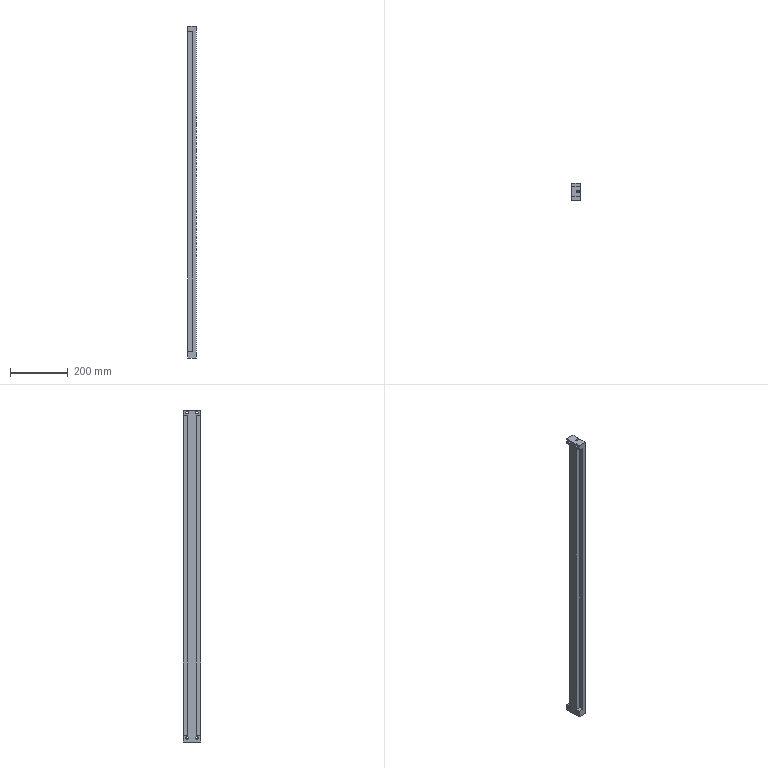Part | STEP file | 750038306 | 1 solid | 26 faces | box 30 x 60 x 1149 mm | volume 1360456 mm3 | plane 18 | cylinder 8 | commonest cylinder face diameters 9 x8
STEP:
#1=CARTESIAN_POINT('',(30.,13.,9.5));
#2=VERTEX_POINT('',#1);
#3=CARTESIAN_POINT('',(30.,13.,18.5));
#4=VERTEX_POINT('',#3);
#5=CARTESIAN_POINT('',(30.,13.,14.));
#6=DIRECTION('',(-1.,0.,0.));
#7=DIRECTION('',(0.,0.,1.));
#8=AXIS2_PLACEMENT_3D('',#5,#6,#7);
#9=CIRCLE('',#8,4.5);
#10=EDGE_CURVE('',#2,#4,#9,.T.);
#11=ORIENTED_EDGE('',*,*,#10,.F.);
#12=CARTESIAN_POINT('',(0.,13.,9.5));
#13=VERTEX_POINT('',#12);
#14=CARTESIAN_POINT('',(33.,13.,9.5));
#15=DIRECTION('',(-1.,0.,0.));
#16=VECTOR('',#15,1000.);
#17=LINE('',#14,#16);
#18=EDGE_CURVE('',#2,#13,#17,.T.);
#19=ORIENTED_EDGE('',*,*,#18,.T.);
#20=CARTESIAN_POINT('',(0.,13.,18.5));
#21=VERTEX_POINT('',#20);
#22=CARTESIAN_POINT('',(0.,13.,14.));
#23=DIRECTION('',(-1.,0.,0.));
#24=DIRECTION('',(0.,0.,1.));
#25=AXIS2_PLACEMENT_3D('',#22,#23,#24);
#26=CIRCLE('',#25,4.5);
#27=EDGE_CURVE('',#13,#21,#26,.T.);
#28=ORIENTED_EDGE('',*,*,#27,.T.);
#29=CARTESIAN_POINT('',(33.,13.,18.5));
#30=DIRECTION('',(-1.,0.,0.));
#31=VECTOR('',#30,1000.);
#32=LINE('',#29,#31);
#33=EDGE_CURVE('',#4,#21,#32,.T.);
#34=ORIENTED_EDGE('',*,*,#33,.F.);
#35=EDGE_LOOP('',(#11,#19,#28,#34));
#36=FACE_OUTER_BOUND('',#35,.T.);
#37=CARTESIAN_POINT('',(33.,13.,14.));
#38=DIRECTION('',(-1.,0.,0.));
#39=DIRECTION('',(0.,0.,1.));
#40=AXIS2_PLACEMENT_3D('',#37,#38,#39);
#41=CYLINDRICAL_SURFACE('',#40,4.5);
#42=ADVANCED_FACE('',(#36),#41,.F.);
#43=CARTESIAN_POINT('',(30.,47.,9.5));
#44=VERTEX_POINT('',#43);
#45=CARTESIAN_POINT('',(30.,47.,18.5));
#46=VERTEX_POINT('',#45);
#47=CARTESIAN_POINT('',(30.,47.,14.));
#48=DIRECTION('',(-1.,0.,0.));
#49=DIRECTION('',(0.,0.,1.));
#50=AXIS2_PLACEMENT_3D('',#47,#48,#49);
#51=CIRCLE('',#50,4.5);
#52=EDGE_CURVE('',#44,#46,#51,.T.);
#53=ORIENTED_EDGE('',*,*,#52,.F.);
#54=CARTESIAN_POINT('',(0.,47.,9.5));
#55=VERTEX_POINT('',#54);
#56=CARTESIAN_POINT('',(33.,47.,9.5));
#57=DIRECTION('',(-1.,0.,0.));
#58=VECTOR('',#57,1000.);
#59=LINE('',#56,#58);
#60=EDGE_CURVE('',#44,#55,#59,.T.);
#61=ORIENTED_EDGE('',*,*,#60,.T.);
#62=CARTESIAN_POINT('',(0.,47.,18.5));
#63=VERTEX_POINT('',#62);
#64=CARTESIAN_POINT('',(0.,47.,14.));
#65=DIRECTION('',(-1.,0.,0.));
#66=DIRECTION('',(0.,0.,1.));
#67=AXIS2_PLACEMENT_3D('',#64,#65,#66);
#68=CIRCLE('',#67,4.5);
#69=EDGE_CURVE('',#55,#63,#68,.T.);
#70=ORIENTED_EDGE('',*,*,#69,.T.);
#71=CARTESIAN_POINT('',(33.,47.,18.5));
#72=DIRECTION('',(-1.,0.,0.));
#73=VECTOR('',#72,1000.);
#74=LINE('',#71,#73);
#75=EDGE_CURVE('',#46,#63,#74,.T.);
#76=ORIENTED_EDGE('',*,*,#75,.F.);
#77=EDGE_LOOP('',(#53,#61,#70,#76));
#78=FACE_OUTER_BOUND('',#77,.T.);
#79=CARTESIAN_POINT('',(33.,47.,14.));
#80=DIRECTION('',(-1.,0.,0.));
#81=DIRECTION('',(0.,0.,1.));
#82=AXIS2_PLACEMENT_3D('',#79,#80,#81);
#83=CYLINDRICAL_SURFACE('',#82,4.5);
#84=ADVANCED_FACE('',(#78),#83,.F.);
#85=CARTESIAN_POINT('',(30.,13.,1135.5));
#86=VERTEX_POINT('',#85);
#87=CARTESIAN_POINT('',(30.,13.,1144.5));
#88=VERTEX_POINT('',#87);
#89=CARTESIAN_POINT('',(30.,13.,1140.));
#90=DIRECTION('',(-1.,0.,0.));
#91=DIRECTION('',(0.,0.,1.));
#92=AXIS2_PLACEMENT_3D('',#89,#90,#91);
#93=CIRCLE('',#92,4.5);
#94=EDGE_CURVE('',#86,#88,#93,.T.);
#95=ORIENTED_EDGE('',*,*,#94,.F.);
#96=CARTESIAN_POINT('',(0.,13.,1135.5));
#97=VERTEX_POINT('',#96);
#98=CARTESIAN_POINT('',(33.,13.,1135.5));
#99=DIRECTION('',(-1.,0.,0.));
#100=VECTOR('',#99,1000.);
#101=LINE('',#98,#100);
#102=EDGE_CURVE('',#86,#97,#101,.T.);
#103=ORIENTED_EDGE('',*,*,#102,.T.);
#104=CARTESIAN_POINT('',(0.,13.,1144.5));
#105=VERTEX_POINT('',#104);
#106=CARTESIAN_POINT('',(0.,13.,1140.));
#107=DIRECTION('',(-1.,0.,0.));
#108=DIRECTION('',(0.,0.,1.));
#109=AXIS2_PLACEMENT_3D('',#106,#107,#108);
#110=CIRCLE('',#109,4.5);
#111=EDGE_CURVE('',#97,#105,#110,.T.);
#112=ORIENTED_EDGE('',*,*,#111,.T.);
#113=CARTESIAN_POINT('',(33.,13.,1144.5));
#114=DIRECTION('',(-1.,0.,0.));
#115=VECTOR('',#114,1000.);
#116=LINE('',#113,#115);
#117=EDGE_CURVE('',#88,#105,#116,.T.);
#118=ORIENTED_EDGE('',*,*,#117,.F.);
#119=EDGE_LOOP('',(#95,#103,#112,#118));
#120=FACE_OUTER_BOUND('',#119,.T.);
#121=CARTESIAN_POINT('',(33.,13.,1140.));
#122=DIRECTION('',(-1.,0.,0.));
#123=DIRECTION('',(0.,0.,1.));
#124=AXIS2_PLACEMENT_3D('',#121,#122,#123);
#125=CYLINDRICAL_SURFACE('',#124,4.5);
#126=ADVANCED_FACE('',(#120),#125,.F.);
#127=CARTESIAN_POINT('',(30.,47.,1135.5));
#128=VERTEX_POINT('',#127);
#129=CARTESIAN_POINT('',(30.,47.,1144.5));
#130=VERTEX_POINT('',#129);
#131=CARTESIAN_POINT('',(30.,47.,1140.));
#132=DIRECTION('',(-1.,0.,0.));
#133=DIRECTION('',(0.,0.,1.));
#134=AXIS2_PLACEMENT_3D('',#131,#132,#133);
#135=CIRCLE('',#134,4.5);
#136=EDGE_CURVE('',#128,#130,#135,.T.);
#137=ORIENTED_EDGE('',*,*,#136,.F.);
#138=CARTESIAN_POINT('',(0.,47.,1135.5));
#139=VERTEX_POINT('',#138);
#140=CARTESIAN_POINT('',(33.,47.,1135.5));
#141=DIRECTION('',(-1.,0.,0.));
#142=VECTOR('',#141,1000.);
#143=LINE('',#140,#142);
#144=EDGE_CURVE('',#128,#139,#143,.T.);
#145=ORIENTED_EDGE('',*,*,#144,.T.);
#146=CARTESIAN_POINT('',(0.,47.,1144.5));
#147=VERTEX_POINT('',#146);
#148=CARTESIAN_POINT('',(0.,47.,1140.));
#149=DIRECTION('',(-1.,0.,0.));
#150=DIRECTION('',(0.,0.,1.));
#151=AXIS2_PLACEMENT_3D('',#148,#149,#150);
#152=CIRCLE('',#151,4.5);
#153=EDGE_CURVE('',#139,#147,#152,.T.);
#154=ORIENTED_EDGE('',*,*,#153,.T.);
#155=CARTESIAN_POINT('',(33.,47.,1144.5));
#156=DIRECTION('',(-1.,0.,0.));
#157=VECTOR('',#156,1000.);
#158=LINE('',#155,#157);
#159=EDGE_CURVE('',#130,#147,#158,.T.);
#160=ORIENTED_EDGE('',*,*,#159,.F.);
#161=EDGE_LOOP('',(#137,#145,#154,#160));
#162=FACE_OUTER_BOUND('',#161,.T.);
#163=CARTESIAN_POINT('',(33.,47.,1140.));
#164=DIRECTION('',(-1.,0.,0.));
#165=DIRECTION('',(0.,0.,1.));
#166=AXIS2_PLACEMENT_3D('',#163,#164,#165);
#167=CYLINDRICAL_SURFACE('',#166,4.5);
#168=ADVANCED_FACE('',(#162),#167,.F.);
#169=CARTESIAN_POINT('',(0.,13.,14.));
#170=DIRECTION('',(-1.,0.,0.));
#171=DIRECTION('',(0.,0.,1.));
#172=AXIS2_PLACEMENT_3D('',#169,#170,#171);
#173=CIRCLE('',#172,4.5);
#174=EDGE_CURVE('',#21,#13,#173,.T.);
#175=ORIENTED_EDGE('',*,*,#174,.F.);
#176=ORIENTED_EDGE('',*,*,#27,.F.);
#177=EDGE_LOOP('',(#175,#176));
#178=FACE_BOUND('',#177,.T.);
#179=CARTESIAN_POINT('',(0.,0.,24.));
#180=VERTEX_POINT('',#179);
#181=CARTESIAN_POINT('',(0.,0.,0.));
#182=VERTEX_POINT('',#181);
#183=CARTESIAN_POINT('',(0.,0.,1149.));
#184=DIRECTION('',(0.,0.,-1.));
#185=VECTOR('',#184,1000.);
#186=LINE('',#183,#185);
#187=EDGE_CURVE('',#180,#182,#186,.T.);
#188=ORIENTED_EDGE('',*,*,#187,.F.);
#189=CARTESIAN_POINT('',(0.,15.,24.));
#190=VERTEX_POINT('',#189);
#191=CARTESIAN_POINT('',(0.,45.,24.));
#192=DIRECTION('',(0.,-1.,0.));
#193=VECTOR('',#192,1000.);
#194=LINE('',#191,#193);
#195=EDGE_CURVE('',#190,#180,#194,.T.);
#196=ORIENTED_EDGE('',*,*,#195,.F.);
#197=CARTESIAN_POINT('',(0.,15.,1129.));
#198=VERTEX_POINT('',#197);
#199=CARTESIAN_POINT('',(0.,15.,1149.));
#200=DIRECTION('',(0.,0.,-1.));
#201=VECTOR('',#200,1000.);
#202=LINE('',#199,#201);
#203=EDGE_CURVE('',#198,#190,#202,.T.);
#204=ORIENTED_EDGE('',*,*,#203,.F.);
#205=CARTESIAN_POINT('',(0.,0.,1129.));
#206=VERTEX_POINT('',#205);
#207=CARTESIAN_POINT('',(0.,45.,1129.));
#208=DIRECTION('',(0.,1.,0.));
#209=VECTOR('',#208,1000.);
#210=LINE('',#207,#209);
#211=EDGE_CURVE('',#206,#198,#210,.T.);
#212=ORIENTED_EDGE('',*,*,#211,.F.);
#213=CARTESIAN_POINT('',(0.,0.,1149.));
#214=VERTEX_POINT('',#213);
#215=CARTESIAN_POINT('',(0.,0.,1149.));
#216=DIRECTION('',(0.,0.,-1.));
#217=VECTOR('',#216,1000.);
#218=LINE('',#215,#217);
#219=EDGE_CURVE('',#214,#206,#218,.T.);
#220=ORIENTED_EDGE('',*,*,#219,.F.);
#221=CARTESIAN_POINT('',(0.,60.,1149.));
#222=VERTEX_POINT('',#221);
#223=CARTESIAN_POINT('',(0.,45.,1149.));
#224=DIRECTION('',(0.,-1.,0.));
#225=VECTOR('',#224,1000.);
#226=LINE('',#223,#225);
#227=EDGE_CURVE('',#222,#214,#226,.T.);
#228=ORIENTED_EDGE('',*,*,#227,.F.);
#229=CARTESIAN_POINT('',(0.,60.,1129.));
#230=VERTEX_POINT('',#229);
#231=CARTESIAN_POINT('',(0.,60.,1149.));
#232=DIRECTION('',(0.,0.,1.));
#233=VECTOR('',#232,1000.);
#234=LINE('',#231,#233);
#235=EDGE_CURVE('',#230,#222,#234,.T.);
#236=ORIENTED_EDGE('',*,*,#235,.F.);
#237=CARTESIAN_POINT('',(0.,45.,1129.));
#238=VERTEX_POINT('',#237);
#239=CARTESIAN_POINT('',(0.,45.,1129.));
#240=DIRECTION('',(0.,1.,0.));
#241=VECTOR('',#240,1000.);
#242=LINE('',#239,#241);
#243=EDGE_CURVE('',#238,#230,#242,.T.);
#244=ORIENTED_EDGE('',*,*,#243,.F.);
#245=CARTESIAN_POINT('',(0.,45.,24.));
#246=VERTEX_POINT('',#245);
#247=CARTESIAN_POINT('',(0.,45.,1149.));
#248=DIRECTION('',(0.,0.,1.));
#249=VECTOR('',#248,1000.);
#250=LINE('',#247,#249);
#251=EDGE_CURVE('',#246,#238,#250,.T.);
#252=ORIENTED_EDGE('',*,*,#251,.F.);
#253=CARTESIAN_POINT('',(0.,60.,24.));
#254=VERTEX_POINT('',#253);
#255=CARTESIAN_POINT('',(0.,45.,24.));
#256=DIRECTION('',(0.,-1.,0.));
#257=VECTOR('',#256,1000.);
#258=LINE('',#255,#257);
#259=EDGE_CURVE('',#254,#246,#258,.T.);
#260=ORIENTED_EDGE('',*,*,#259,.F.);
#261=CARTESIAN_POINT('',(0.,60.,0.));
#262=VERTEX_POINT('',#261);
#263=CARTESIAN_POINT('',(0.,60.,1149.));
#264=DIRECTION('',(0.,0.,1.));
#265=VECTOR('',#264,1000.);
#266=LINE('',#263,#265);
#267=EDGE_CURVE('',#262,#254,#266,.T.);
#268=ORIENTED_EDGE('',*,*,#267,.F.);
#269=CARTESIAN_POINT('',(0.,45.,0.));
#270=DIRECTION('',(0.,1.,0.));
#271=VECTOR('',#270,1000.);
#272=LINE('',#269,#271);
#273=EDGE_CURVE('',#182,#262,#272,.T.);
#274=ORIENTED_EDGE('',*,*,#273,.F.);
#275=EDGE_LOOP('',(#188,#196,#204,#212,#220,#228,#236,#244,#252,#260,#268,#274));
#276=FACE_OUTER_BOUND('',#275,.T.);
#277=CARTESIAN_POINT('',(0.,47.,14.));
#278=DIRECTION('',(-1.,0.,0.));
#279=DIRECTION('',(0.,0.,1.));
#280=AXIS2_PLACEMENT_3D('',#277,#278,#279);
#281=CIRCLE('',#280,4.5);
#282=EDGE_CURVE('',#63,#55,#281,.T.);
#283=ORIENTED_EDGE('',*,*,#282,.F.);
#284=ORIENTED_EDGE('',*,*,#69,.F.);
#285=EDGE_LOOP('',(#283,#284));
#286=FACE_BOUND('',#285,.T.);
#287=CARTESIAN_POINT('',(0.,13.,1140.));
#288=DIRECTION('',(-1.,0.,0.));
#289=DIRECTION('',(0.,0.,1.));
#290=AXIS2_PLACEMENT_3D('',#287,#288,#289);
#291=CIRCLE('',#290,4.5);
#292=EDGE_CURVE('',#105,#97,#291,.T.);
#293=ORIENTED_EDGE('',*,*,#292,.F.);
#294=ORIENTED_EDGE('',*,*,#111,.F.);
#295=EDGE_LOOP('',(#293,#294));
#296=FACE_BOUND('',#295,.T.);
#297=CARTESIAN_POINT('',(0.,47.,1140.));
#298=DIRECTION('',(-1.,0.,0.));
#299=DIRECTION('',(0.,0.,1.));
#300=AXIS2_PLACEMENT_3D('',#297,#298,#299);
#301=CIRCLE('',#300,4.5);
#302=EDGE_CURVE('',#147,#139,#301,.T.);
#303=ORIENTED_EDGE('',*,*,#302,.F.);
#304=ORIENTED_EDGE('',*,*,#153,.F.);
#305=EDGE_LOOP('',(#303,#304));
#306=FACE_BOUND('',#305,.T.);
#307=CARTESIAN_POINT('',(0.,45.,1149.));
#308=DIRECTION('',(1.,0.,0.));
#309=DIRECTION('',(0.,1.,0.));
#310=AXIS2_PLACEMENT_3D('',#307,#308,#309);
#311=PLANE('',#310);
#312=ADVANCED_FACE('',(#178,#276,#286,#296,#306),#311,.F.);
#313=ORIENTED_EDGE('',*,*,#18,.F.);
#314=CARTESIAN_POINT('',(30.,13.,14.));
#315=DIRECTION('',(-1.,0.,0.));
#316=DIRECTION('',(0.,0.,1.));
#317=AXIS2_PLACEMENT_3D('',#314,#315,#316);
#318=CIRCLE('',#317,4.5);
#319=EDGE_CURVE('',#4,#2,#318,.T.);
#320=ORIENTED_EDGE('',*,*,#319,.F.);
#321=ORIENTED_EDGE('',*,*,#33,.T.);
#322=ORIENTED_EDGE('',*,*,#174,.T.);
#323=EDGE_LOOP('',(#313,#320,#321,#322));
#324=FACE_OUTER_BOUND('',#323,.T.);
#325=CARTESIAN_POINT('',(33.,13.,14.));
#326=DIRECTION('',(-1.,0.,0.));
#327=DIRECTION('',(0.,0.,1.));
#328=AXIS2_PLACEMENT_3D('',#325,#326,#327);
#329=CYLINDRICAL_SURFACE('',#328,4.5);
#330=ADVANCED_FACE('',(#324),#329,.F.);
#331=CARTESIAN_POINT('',(15.,33.,0.));
#332=VERTEX_POINT('',#331);
#333=CARTESIAN_POINT('',(30.,33.,0.));
#334=VERTEX_POINT('',#333);
#335=CARTESIAN_POINT('',(0.,33.,0.));
#336=DIRECTION('',(1.,0.,0.));
#337=VECTOR('',#336,1000.);
#338=LINE('',#335,#337);
#339=EDGE_CURVE('',#332,#334,#338,.T.);
#340=ORIENTED_EDGE('',*,*,#339,.F.);
#341=CARTESIAN_POINT('',(15.,27.,0.));
#342=VERTEX_POINT('',#341);
#343=CARTESIAN_POINT('',(15.,0.,0.));
#344=DIRECTION('',(0.,1.,0.));
#345=VECTOR('',#344,1000.);
#346=LINE('',#343,#345);
#347=EDGE_CURVE('',#342,#332,#346,.T.);
#348=ORIENTED_EDGE('',*,*,#347,.F.);
#349=CARTESIAN_POINT('',(30.,27.,0.));
#350=VERTEX_POINT('',#349);
#351=CARTESIAN_POINT('',(0.,27.,0.));
#352=DIRECTION('',(-1.,0.,0.));
#353=VECTOR('',#352,1000.);
#354=LINE('',#351,#353);
#355=EDGE_CURVE('',#350,#342,#354,.T.);
#356=ORIENTED_EDGE('',*,*,#355,.F.);
#357=CARTESIAN_POINT('',(30.,0.,0.));
#358=VERTEX_POINT('',#357);
#359=CARTESIAN_POINT('',(30.,0.,0.));
#360=DIRECTION('',(0.,1.,0.));
#361=VECTOR('',#360,1000.);
#362=LINE('',#359,#361);
#363=EDGE_CURVE('',#358,#350,#362,.T.);
#364=ORIENTED_EDGE('',*,*,#363,.F.);
#365=CARTESIAN_POINT('',(0.,0.,0.));
#366=DIRECTION('',(1.,0.,0.));
#367=VECTOR('',#366,1000.);
#368=LINE('',#365,#367);
#369=EDGE_CURVE('',#182,#358,#368,.T.);
#370=ORIENTED_EDGE('',*,*,#369,.F.);
#371=ORIENTED_EDGE('',*,*,#273,.T.);
#372=CARTESIAN_POINT('',(30.,60.,0.));
#373=VERTEX_POINT('',#372);
#374=CARTESIAN_POINT('',(0.,60.,0.));
#375=DIRECTION('',(-1.,0.,0.));
#376=VECTOR('',#375,1000.);
#377=LINE('',#374,#376);
#378=EDGE_CURVE('',#373,#262,#377,.T.);
#379=ORIENTED_EDGE('',*,*,#378,.F.);
#380=CARTESIAN_POINT('',(30.,0.,0.));
#381=DIRECTION('',(0.,1.,0.));
#382=VECTOR('',#381,1000.);
#383=LINE('',#380,#382);
#384=EDGE_CURVE('',#334,#373,#383,.T.);
#385=ORIENTED_EDGE('',*,*,#384,.F.);
#386=EDGE_LOOP('',(#340,#348,#356,#364,#370,#371,#379,#385));
#387=FACE_OUTER_BOUND('',#386,.T.);
#388=CARTESIAN_POINT('',(0.,0.,0.));
#389=DIRECTION('',(0.,0.,1.));
#390=DIRECTION('',(1.,0.,0.));
#391=AXIS2_PLACEMENT_3D('',#388,#389,#390);
#392=PLANE('',#391);
#393=ADVANCED_FACE('',(#387),#392,.F.);
#394=CARTESIAN_POINT('',(30.,0.,1149.));
#395=VERTEX_POINT('',#394);
#396=CARTESIAN_POINT('',(30.,0.,1149.));
#397=DIRECTION('',(0.,0.,-1.));
#398=VECTOR('',#397,1000.);
#399=LINE('',#396,#398);
#400=EDGE_CURVE('',#395,#358,#399,.T.);
#401=ORIENTED_EDGE('',*,*,#400,.F.);
#402=CARTESIAN_POINT('',(18.,0.,1149.));
#403=DIRECTION('',(1.,0.,0.));
#404=VECTOR('',#403,1000.);
#405=LINE('',#402,#404);
#406=EDGE_CURVE('',#214,#395,#405,.T.);
#407=ORIENTED_EDGE('',*,*,#406,.F.);
#408=ORIENTED_EDGE('',*,*,#219,.T.);
#409=CARTESIAN_POINT('',(18.,0.,1129.));
#410=VERTEX_POINT('',#409);
#411=CARTESIAN_POINT('',(18.,0.,1129.));
#412=DIRECTION('',(-1.,0.,0.));
#413=VECTOR('',#412,1000.);
#414=LINE('',#411,#413);
#415=EDGE_CURVE('',#410,#206,#414,.T.);
#416=ORIENTED_EDGE('',*,*,#415,.F.);
#417=CARTESIAN_POINT('',(18.,0.,24.));
#418=VERTEX_POINT('',#417);
#419=CARTESIAN_POINT('',(18.,0.,1149.));
#420=DIRECTION('',(0.,0.,1.));
#421=VECTOR('',#420,1000.);
#422=LINE('',#419,#421);
#423=EDGE_CURVE('',#418,#410,#422,.T.);
#424=ORIENTED_EDGE('',*,*,#423,.F.);
#425=CARTESIAN_POINT('',(18.,0.,24.));
#426=DIRECTION('',(1.,0.,0.));
#427=VECTOR('',#426,1000.);
#428=LINE('',#425,#427);
#429=EDGE_CURVE('',#180,#418,#428,.T.);
#430=ORIENTED_EDGE('',*,*,#429,.F.);
#431=ORIENTED_EDGE('',*,*,#187,.T.);
#432=ORIENTED_EDGE('',*,*,#369,.T.);
#433=EDGE_LOOP('',(#401,#407,#408,#416,#424,#430,#431,#432));
#434=FACE_OUTER_BOUND('',#433,.T.);
#435=CARTESIAN_POINT('',(18.,0.,1149.));
#436=DIRECTION('',(0.,1.,0.));
#437=DIRECTION('',(0.,0.,1.));
#438=AXIS2_PLACEMENT_3D('',#435,#436,#437);
#439=PLANE('',#438);
#440=ADVANCED_FACE('',(#434),#439,.F.);
#441=CARTESIAN_POINT('',(18.,15.,24.));
#442=VERTEX_POINT('',#441);
#443=CARTESIAN_POINT('',(33.,15.,24.));
#444=DIRECTION('',(-1.,0.,0.));
#445=VECTOR('',#444,1000.);
#446=LINE('',#443,#445);
#447=EDGE_CURVE('',#442,#190,#446,.T.);
#448=ORIENTED_EDGE('',*,*,#447,.T.);
#449=ORIENTED_EDGE('',*,*,#195,.T.);
#450=ORIENTED_EDGE('',*,*,#429,.T.);
#451=CARTESIAN_POINT('',(18.,0.,24.));
#452=DIRECTION('',(0.,1.,0.));
#453=VECTOR('',#452,1000.);
#454=LINE('',#451,#453);
#455=EDGE_CURVE('',#418,#442,#454,.T.);
#456=ORIENTED_EDGE('',*,*,#455,.T.);
#457=EDGE_LOOP('',(#448,#449,#450,#456));
#458=FACE_OUTER_BOUND('',#457,.T.);
#459=CARTESIAN_POINT('',(33.,0.,24.));
#460=DIRECTION('',(0.,0.,1.));
#461=DIRECTION('',(1.,0.,0.));
#462=AXIS2_PLACEMENT_3D('',#459,#460,#461);
#463=PLANE('',#462);
#464=ADVANCED_FACE('',(#458),#463,.T.);
#465=CARTESIAN_POINT('',(18.,15.,1129.));
#466=VERTEX_POINT('',#465);
#467=CARTESIAN_POINT('',(0.,15.,1129.));
#468=DIRECTION('',(1.,0.,0.));
#469=VECTOR('',#468,1000.);
#470=LINE('',#467,#469);
#471=EDGE_CURVE('',#198,#466,#470,.T.);
#472=ORIENTED_EDGE('',*,*,#471,.F.);
#473=ORIENTED_EDGE('',*,*,#203,.T.);
#474=ORIENTED_EDGE('',*,*,#447,.F.);
#475=CARTESIAN_POINT('',(18.,15.,1149.));
#476=DIRECTION('',(0.,0.,-1.));
#477=VECTOR('',#476,1000.);
#478=LINE('',#475,#477);
#479=EDGE_CURVE('',#466,#442,#478,.T.);
#480=ORIENTED_EDGE('',*,*,#479,.F.);
#481=EDGE_LOOP('',(#472,#473,#474,#480));
#482=FACE_OUTER_BOUND('',#481,.T.);
#483=CARTESIAN_POINT('',(0.,15.,1149.));
#484=DIRECTION('',(0.,1.,0.));
#485=DIRECTION('',(-1.,0.,0.));
#486=AXIS2_PLACEMENT_3D('',#483,#484,#485);
#487=PLANE('',#486);
#488=ADVANCED_FACE('',(#482),#487,.F.);
#489=ORIENTED_EDGE('',*,*,#415,.T.);
#490=ORIENTED_EDGE('',*,*,#211,.T.);
#491=ORIENTED_EDGE('',*,*,#471,.T.);
#492=CARTESIAN_POINT('',(18.,15.,1129.));
#493=DIRECTION('',(0.,-1.,0.));
#494=VECTOR('',#493,1000.);
#495=LINE('',#492,#494);
#496=EDGE_CURVE('',#466,#410,#495,.T.);
#497=ORIENTED_EDGE('',*,*,#496,.T.);
#498=EDGE_LOOP('',(#489,#490,#491,#497));
#499=FACE_OUTER_BOUND('',#498,.T.);
#500=CARTESIAN_POINT('',(33.,15.,1129.));
#501=DIRECTION('',(0.,0.,-1.));
#502=DIRECTION('',(-1.,0.,0.));
#503=AXIS2_PLACEMENT_3D('',#500,#501,#502);
#504=PLANE('',#503);
#505=ADVANCED_FACE('',(#499),#504,.T.);
#506=CARTESIAN_POINT('',(15.,27.,1149.));
#507=VERTEX_POINT('',#506);
#508=CARTESIAN_POINT('',(15.,33.,1149.));
#509=VERTEX_POINT('',#508);
#510=CARTESIAN_POINT('',(15.,0.,1149.));
#511=DIRECTION('',(0.,1.,0.));
#512=VECTOR('',#511,1000.);
#513=LINE('',#510,#512);
#514=EDGE_CURVE('',#507,#509,#513,.T.);
#515=ORIENTED_EDGE('',*,*,#514,.T.);
#516=CARTESIAN_POINT('',(30.,33.,1149.));
#517=VERTEX_POINT('',#516);
#518=CARTESIAN_POINT('',(0.,33.,1149.));
#519=DIRECTION('',(1.,0.,0.));
#520=VECTOR('',#519,1000.);
#521=LINE('',#518,#520);
#522=EDGE_CURVE('',#509,#517,#521,.T.);
#523=ORIENTED_EDGE('',*,*,#522,.T.);
#524=CARTESIAN_POINT('',(30.,60.,1149.));
#525=VERTEX_POINT('',#524);
#526=CARTESIAN_POINT('',(30.,0.,1149.));
#527=DIRECTION('',(0.,1.,0.));
#528=VECTOR('',#527,1000.);
#529=LINE('',#526,#528);
#530=EDGE_CURVE('',#517,#525,#529,.T.);
#531=ORIENTED_EDGE('',*,*,#530,.T.);
#532=CARTESIAN_POINT('',(0.,60.,1149.));
#533=DIRECTION('',(-1.,0.,0.));
#534=VECTOR('',#533,1000.);
#535=LINE('',#532,#534);
#536=EDGE_CURVE('',#525,#222,#535,.T.);
#537=ORIENTED_EDGE('',*,*,#536,.T.);
#538=ORIENTED_EDGE('',*,*,#227,.T.);
#539=ORIENTED_EDGE('',*,*,#406,.T.);
#540=CARTESIAN_POINT('',(30.,27.,1149.));
#541=VERTEX_POINT('',#540);
#542=CARTESIAN_POINT('',(30.,0.,1149.));
#543=DIRECTION('',(0.,1.,0.));
#544=VECTOR('',#543,1000.);
#545=LINE('',#542,#544);
#546=EDGE_CURVE('',#395,#541,#545,.T.);
#547=ORIENTED_EDGE('',*,*,#546,.T.);
#548=CARTESIAN_POINT('',(0.,27.,1149.));
#549=DIRECTION('',(-1.,0.,0.));
#550=VECTOR('',#549,1000.);
#551=LINE('',#548,#550);
#552=EDGE_CURVE('',#541,#507,#551,.T.);
#553=ORIENTED_EDGE('',*,*,#552,.T.);
#554=EDGE_LOOP('',(#515,#523,#531,#537,#538,#539,#547,#553));
#555=FACE_OUTER_BOUND('',#554,.T.);
#556=CARTESIAN_POINT('',(0.,0.,1149.));
#557=DIRECTION('',(0.,0.,1.));
#558=DIRECTION('',(1.,0.,0.));
#559=AXIS2_PLACEMENT_3D('',#556,#557,#558);
#560=PLANE('',#559);
#561=ADVANCED_FACE('',(#555),#560,.T.);
#562=ORIENTED_EDGE('',*,*,#267,.T.);
#563=CARTESIAN_POINT('',(18.,60.,24.));
#564=VERTEX_POINT('',#563);
#565=CARTESIAN_POINT('',(30.,60.,24.));
#566=DIRECTION('',(-1.,0.,0.));
#567=VECTOR('',#566,1000.);
#568=LINE('',#565,#567);
#569=EDGE_CURVE('',#564,#254,#568,.T.);
#570=ORIENTED_EDGE('',*,*,#569,.F.);
#571=CARTESIAN_POINT('',(18.,60.,1129.));
#572=VERTEX_POINT('',#571);
#573=CARTESIAN_POINT('',(18.,60.,1149.));
#574=DIRECTION('',(0.,0.,-1.));
#575=VECTOR('',#574,1000.);
#576=LINE('',#573,#575);
#577=EDGE_CURVE('',#572,#564,#576,.T.);
#578=ORIENTED_EDGE('',*,*,#577,.F.);
#579=CARTESIAN_POINT('',(30.,60.,1129.));
#580=DIRECTION('',(1.,0.,0.));
#581=VECTOR('',#580,1000.);
#582=LINE('',#579,#581);
#583=EDGE_CURVE('',#230,#572,#582,.T.);
#584=ORIENTED_EDGE('',*,*,#583,.F.);
#585=ORIENTED_EDGE('',*,*,#235,.T.);
#586=ORIENTED_EDGE('',*,*,#536,.F.);
#587=CARTESIAN_POINT('',(30.,60.,1149.));
#588=DIRECTION('',(0.,0.,1.));
#589=VECTOR('',#588,1000.);
#590=LINE('',#587,#589);
#591=EDGE_CURVE('',#373,#525,#590,.T.);
#592=ORIENTED_EDGE('',*,*,#591,.F.);
#593=ORIENTED_EDGE('',*,*,#378,.T.);
#594=EDGE_LOOP('',(#562,#570,#578,#584,#585,#586,#592,#593));
#595=FACE_OUTER_BOUND('',#594,.T.);
#596=CARTESIAN_POINT('',(30.,60.,1149.));
#597=DIRECTION('',(0.,-1.,0.));
#598=DIRECTION('',(0.,0.,-1.));
#599=AXIS2_PLACEMENT_3D('',#596,#597,#598);
#600=PLANE('',#599);
#601=ADVANCED_FACE('',(#595),#600,.F.);
#602=CARTESIAN_POINT('',(18.,45.,1129.));
#603=VERTEX_POINT('',#602);
#604=CARTESIAN_POINT('',(33.,45.,1129.));
#605=DIRECTION('',(-1.,0.,0.));
#606=VECTOR('',#605,1000.);
#607=LINE('',#604,#606);
#608=EDGE_CURVE('',#603,#238,#607,.T.);
#609=ORIENTED_EDGE('',*,*,#608,.T.);
#610=ORIENTED_EDGE('',*,*,#243,.T.);
#611=ORIENTED_EDGE('',*,*,#583,.T.);
#612=CARTESIAN_POINT('',(18.,60.,1129.));
#613=DIRECTION('',(0.,-1.,0.));
#614=VECTOR('',#613,1000.);
#615=LINE('',#612,#614);
#616=EDGE_CURVE('',#572,#603,#615,.T.);
#617=ORIENTED_EDGE('',*,*,#616,.T.);
#618=EDGE_LOOP('',(#609,#610,#611,#617));
#619=FACE_OUTER_BOUND('',#618,.T.);
#620=CARTESIAN_POINT('',(33.,60.,1129.));
#621=DIRECTION('',(0.,0.,-1.));
#622=DIRECTION('',(-1.,0.,0.));
#623=AXIS2_PLACEMENT_3D('',#620,#621,#622);
#624=PLANE('',#623);
#625=ADVANCED_FACE('',(#619),#624,.T.);
#626=CARTESIAN_POINT('',(18.,45.,24.));
#627=VERTEX_POINT('',#626);
#628=CARTESIAN_POINT('',(18.,45.,1149.));
#629=DIRECTION('',(0.,0.,1.));
#630=VECTOR('',#629,1000.);
#631=LINE('',#628,#630);
#632=EDGE_CURVE('',#627,#603,#631,.T.);
#633=ORIENTED_EDGE('',*,*,#632,.F.);
#634=CARTESIAN_POINT('',(18.,45.,24.));
#635=DIRECTION('',(1.,0.,0.));
#636=VECTOR('',#635,1000.);
#637=LINE('',#634,#636);
#638=EDGE_CURVE('',#246,#627,#637,.T.);
#639=ORIENTED_EDGE('',*,*,#638,.F.);
#640=ORIENTED_EDGE('',*,*,#251,.T.);
#641=ORIENTED_EDGE('',*,*,#608,.F.);
#642=EDGE_LOOP('',(#633,#639,#640,#641));
#643=FACE_OUTER_BOUND('',#642,.T.);
#644=CARTESIAN_POINT('',(18.,45.,1149.));
#645=DIRECTION('',(0.,-1.,0.));
#646=DIRECTION('',(1.,0.,0.));
#647=AXIS2_PLACEMENT_3D('',#644,#645,#646);
#648=PLANE('',#647);
#649=ADVANCED_FACE('',(#643),#648,.F.);
#650=ORIENTED_EDGE('',*,*,#569,.T.);
#651=ORIENTED_EDGE('',*,*,#259,.T.);
#652=ORIENTED_EDGE('',*,*,#638,.T.);
#653=CARTESIAN_POINT('',(18.,45.,24.));
#654=DIRECTION('',(0.,1.,0.));
#655=VECTOR('',#654,1000.);
#656=LINE('',#653,#655);
#657=EDGE_CURVE('',#627,#564,#656,.T.);
#658=ORIENTED_EDGE('',*,*,#657,.T.);
#659=EDGE_LOOP('',(#650,#651,#652,#658));
#660=FACE_OUTER_BOUND('',#659,.T.);
#661=CARTESIAN_POINT('',(33.,45.,24.));
#662=DIRECTION('',(0.,0.,1.));
#663=DIRECTION('',(1.,0.,0.));
#664=AXIS2_PLACEMENT_3D('',#661,#662,#663);
#665=PLANE('',#664);
#666=ADVANCED_FACE('',(#660),#665,.T.);
#667=ORIENTED_EDGE('',*,*,#60,.F.);
#668=CARTESIAN_POINT('',(30.,47.,14.));
#669=DIRECTION('',(-1.,0.,0.));
#670=DIRECTION('',(0.,0.,1.));
#671=AXIS2_PLACEMENT_3D('',#668,#669,#670);
#672=CIRCLE('',#671,4.5);
#673=EDGE_CURVE('',#46,#44,#672,.T.);
#674=ORIENTED_EDGE('',*,*,#673,.F.);
#675=ORIENTED_EDGE('',*,*,#75,.T.);
#676=ORIENTED_EDGE('',*,*,#282,.T.);
#677=EDGE_LOOP('',(#667,#674,#675,#676));
#678=FACE_OUTER_BOUND('',#677,.T.);
#679=CARTESIAN_POINT('',(33.,47.,14.));
#680=DIRECTION('',(-1.,0.,0.));
#681=DIRECTION('',(0.,0.,1.));
#682=AXIS2_PLACEMENT_3D('',#679,#680,#681);
#683=CYLINDRICAL_SURFACE('',#682,4.5);
#684=ADVANCED_FACE('',(#678),#683,.F.);
#685=ORIENTED_EDGE('',*,*,#102,.F.);
#686=CARTESIAN_POINT('',(30.,13.,1140.));
#687=DIRECTION('',(-1.,0.,0.));
#688=DIRECTION('',(0.,0.,1.));
#689=AXIS2_PLACEMENT_3D('',#686,#687,#688);
#690=CIRCLE('',#689,4.5);
#691=EDGE_CURVE('',#88,#86,#690,.T.);
#692=ORIENTED_EDGE('',*,*,#691,.F.);
#693=ORIENTED_EDGE('',*,*,#117,.T.);
#694=ORIENTED_EDGE('',*,*,#292,.T.);
#695=EDGE_LOOP('',(#685,#692,#693,#694));
#696=FACE_OUTER_BOUND('',#695,.T.);
#697=CARTESIAN_POINT('',(33.,13.,1140.));
#698=DIRECTION('',(-1.,0.,0.));
#699=DIRECTION('',(0.,0.,1.));
#700=AXIS2_PLACEMENT_3D('',#697,#698,#699);
#701=CYLINDRICAL_SURFACE('',#700,4.5);
#702=ADVANCED_FACE('',(#696),#701,.F.);
#703=ORIENTED_EDGE('',*,*,#144,.F.);
#704=CARTESIAN_POINT('',(30.,47.,1140.));
#705=DIRECTION('',(-1.,0.,0.));
#706=DIRECTION('',(0.,0.,1.));
#707=AXIS2_PLACEMENT_3D('',#704,#705,#706);
#708=CIRCLE('',#707,4.5);
#709=EDGE_CURVE('',#130,#128,#708,.T.);
#710=ORIENTED_EDGE('',*,*,#709,.F.);
#711=ORIENTED_EDGE('',*,*,#159,.T.);
#712=ORIENTED_EDGE('',*,*,#302,.T.);
#713=EDGE_LOOP('',(#703,#710,#711,#712));
#714=FACE_OUTER_BOUND('',#713,.T.);
#715=CARTESIAN_POINT('',(33.,47.,1140.));
#716=DIRECTION('',(-1.,0.,0.));
#717=DIRECTION('',(0.,0.,1.));
#718=AXIS2_PLACEMENT_3D('',#715,#716,#717);
#719=CYLINDRICAL_SURFACE('',#718,4.5);
#720=ADVANCED_FACE('',(#714),#719,.F.);
#721=CARTESIAN_POINT('',(30.,27.,1149.));
#722=DIRECTION('',(0.,0.,-1.));
#723=VECTOR('',#722,1000.);
#724=LINE('',#721,#723);
#725=EDGE_CURVE('',#541,#350,#724,.T.);
#726=ORIENTED_EDGE('',*,*,#725,.F.);
#727=ORIENTED_EDGE('',*,*,#546,.F.);
#728=ORIENTED_EDGE('',*,*,#400,.T.);
#729=ORIENTED_EDGE('',*,*,#363,.T.);
#730=EDGE_LOOP('',(#726,#727,#728,#729));
#731=FACE_OUTER_BOUND('',#730,.T.);
#732=ORIENTED_EDGE('',*,*,#691,.T.);
#733=ORIENTED_EDGE('',*,*,#94,.T.);
#734=EDGE_LOOP('',(#732,#733));
#735=FACE_BOUND('',#734,.T.);
#736=ORIENTED_EDGE('',*,*,#319,.T.);
#737=ORIENTED_EDGE('',*,*,#10,.T.);
#738=EDGE_LOOP('',(#736,#737));
#739=FACE_BOUND('',#738,.T.);
#740=CARTESIAN_POINT('',(30.,0.,1149.));
#741=DIRECTION('',(-1.,0.,0.));
#742=DIRECTION('',(0.,-1.,0.));
#743=AXIS2_PLACEMENT_3D('',#740,#741,#742);
#744=PLANE('',#743);
#745=ADVANCED_FACE('',(#731,#735,#739),#744,.F.);
#746=ORIENTED_EDGE('',*,*,#591,.T.);
#747=ORIENTED_EDGE('',*,*,#530,.F.);
#748=CARTESIAN_POINT('',(30.,33.,1149.));
#749=DIRECTION('',(0.,0.,1.));
#750=VECTOR('',#749,1000.);
#751=LINE('',#748,#750);
#752=EDGE_CURVE('',#334,#517,#751,.T.);
#753=ORIENTED_EDGE('',*,*,#752,.F.);
#754=ORIENTED_EDGE('',*,*,#384,.T.);
#755=EDGE_LOOP('',(#746,#747,#753,#754));
#756=FACE_OUTER_BOUND('',#755,.T.);
#757=ORIENTED_EDGE('',*,*,#673,.T.);
#758=ORIENTED_EDGE('',*,*,#52,.T.);
#759=EDGE_LOOP('',(#757,#758));
#760=FACE_BOUND('',#759,.T.);
#761=ORIENTED_EDGE('',*,*,#709,.T.);
#762=ORIENTED_EDGE('',*,*,#136,.T.);
#763=EDGE_LOOP('',(#761,#762));
#764=FACE_BOUND('',#763,.T.);
#765=CARTESIAN_POINT('',(30.,33.,1149.));
#766=DIRECTION('',(-1.,0.,0.));
#767=DIRECTION('',(0.,0.,1.));
#768=AXIS2_PLACEMENT_3D('',#765,#766,#767);
#769=PLANE('',#768);
#770=ADVANCED_FACE('',(#756,#760,#764),#769,.F.);
#771=ORIENTED_EDGE('',*,*,#752,.T.);
#772=ORIENTED_EDGE('',*,*,#522,.F.);
#773=CARTESIAN_POINT('',(15.,33.,1149.));
#774=DIRECTION('',(0.,0.,1.));
#775=VECTOR('',#774,1000.);
#776=LINE('',#773,#775);
#777=EDGE_CURVE('',#332,#509,#776,.T.);
#778=ORIENTED_EDGE('',*,*,#777,.F.);
#779=ORIENTED_EDGE('',*,*,#339,.T.);
#780=EDGE_LOOP('',(#771,#772,#778,#779));
#781=FACE_OUTER_BOUND('',#780,.T.);
#782=CARTESIAN_POINT('',(15.,33.,1149.));
#783=DIRECTION('',(0.,1.,0.));
#784=DIRECTION('',(0.,0.,1.));
#785=AXIS2_PLACEMENT_3D('',#782,#783,#784);
#786=PLANE('',#785);
#787=ADVANCED_FACE('',(#781),#786,.F.);
#788=ORIENTED_EDGE('',*,*,#777,.T.);
#789=ORIENTED_EDGE('',*,*,#514,.F.);
#790=CARTESIAN_POINT('',(15.,27.,1149.));
#791=DIRECTION('',(0.,0.,1.));
#792=VECTOR('',#791,1000.);
#793=LINE('',#790,#792);
#794=EDGE_CURVE('',#342,#507,#793,.T.);
#795=ORIENTED_EDGE('',*,*,#794,.F.);
#796=ORIENTED_EDGE('',*,*,#347,.T.);
#797=EDGE_LOOP('',(#788,#789,#795,#796));
#798=FACE_OUTER_BOUND('',#797,.T.);
#799=CARTESIAN_POINT('',(15.,27.,1149.));
#800=DIRECTION('',(-1.,0.,0.));
#801=DIRECTION('',(0.,0.,1.));
#802=AXIS2_PLACEMENT_3D('',#799,#800,#801);
#803=PLANE('',#802);
#804=ADVANCED_FACE('',(#798),#803,.F.);
#805=ORIENTED_EDGE('',*,*,#794,.T.);
#806=ORIENTED_EDGE('',*,*,#552,.F.);
#807=ORIENTED_EDGE('',*,*,#725,.T.);
#808=ORIENTED_EDGE('',*,*,#355,.T.);
#809=EDGE_LOOP('',(#805,#806,#807,#808));
#810=FACE_OUTER_BOUND('',#809,.T.);
#811=CARTESIAN_POINT('',(30.,27.,1149.));
#812=DIRECTION('',(0.,-1.,0.));
#813=DIRECTION('',(0.,0.,-1.));
#814=AXIS2_PLACEMENT_3D('',#811,#812,#813);
#815=PLANE('',#814);
#816=ADVANCED_FACE('',(#810),#815,.F.);
#817=ORIENTED_EDGE('',*,*,#479,.T.);
#818=ORIENTED_EDGE('',*,*,#455,.F.);
#819=ORIENTED_EDGE('',*,*,#423,.T.);
#820=ORIENTED_EDGE('',*,*,#496,.F.);
#821=EDGE_LOOP('',(#817,#818,#819,#820));
#822=FACE_OUTER_BOUND('',#821,.T.);
#823=CARTESIAN_POINT('',(18.,15.,1149.));
#824=DIRECTION('',(1.,0.,0.));
#825=DIRECTION('',(0.,1.,0.));
#826=AXIS2_PLACEMENT_3D('',#823,#824,#825);
#827=PLANE('',#826);
#828=ADVANCED_FACE('',(#822),#827,.F.);
#829=ORIENTED_EDGE('',*,*,#577,.T.);
#830=ORIENTED_EDGE('',*,*,#657,.F.);
#831=ORIENTED_EDGE('',*,*,#632,.T.);
#832=ORIENTED_EDGE('',*,*,#616,.F.);
#833=EDGE_LOOP('',(#829,#830,#831,#832));
#834=FACE_OUTER_BOUND('',#833,.T.);
#835=CARTESIAN_POINT('',(18.,60.,1149.));
#836=DIRECTION('',(1.,0.,0.));
#837=DIRECTION('',(0.,1.,0.));
#838=AXIS2_PLACEMENT_3D('',#835,#836,#837);
#839=PLANE('',#838);
#840=ADVANCED_FACE('',(#834),#839,.F.);
#841=CLOSED_SHELL('',(#42,#84,#126,#168,#312,#330,#393,#440,#464,#488,#505,#561,#601,#625,#649,#666,#684,#702,#720,#745,#770,#787,#804,#816,#828,#840));
#842=MANIFOLD_SOLID_BREP('',#841);
#843=CARTESIAN_POINT('',(0.,0.,0.));
#844=DIRECTION('',(0.,0.,1.));
#845=DIRECTION('',(1.,0.,0.));
#846=AXIS2_PLACEMENT_3D('',#843,#844,#845);
#847=(LENGTH_UNIT()NAMED_UNIT(*)SI_UNIT(.MILLI.,.METRE.));
#848=UNCERTAINTY_MEASURE_WITH_UNIT(LENGTH_MEASURE(0.00001),#847,'','');
#849=(NAMED_UNIT(*)PLANE_ANGLE_UNIT()SI_UNIT($,.RADIAN.));
#850=(NAMED_UNIT(*)SI_UNIT($,.STERADIAN.)SOLID_ANGLE_UNIT());
#851=(GEOMETRIC_REPRESENTATION_CONTEXT(3)GLOBAL_UNCERTAINTY_ASSIGNED_CONTEXT((#848))GLOBAL_UNIT_ASSIGNED_CONTEXT((#847,#849,#850))REPRESENTATION_CONTEXT('',''));
#852=ADVANCED_BREP_SHAPE_REPRESENTATION('',(#842,#846),#851);